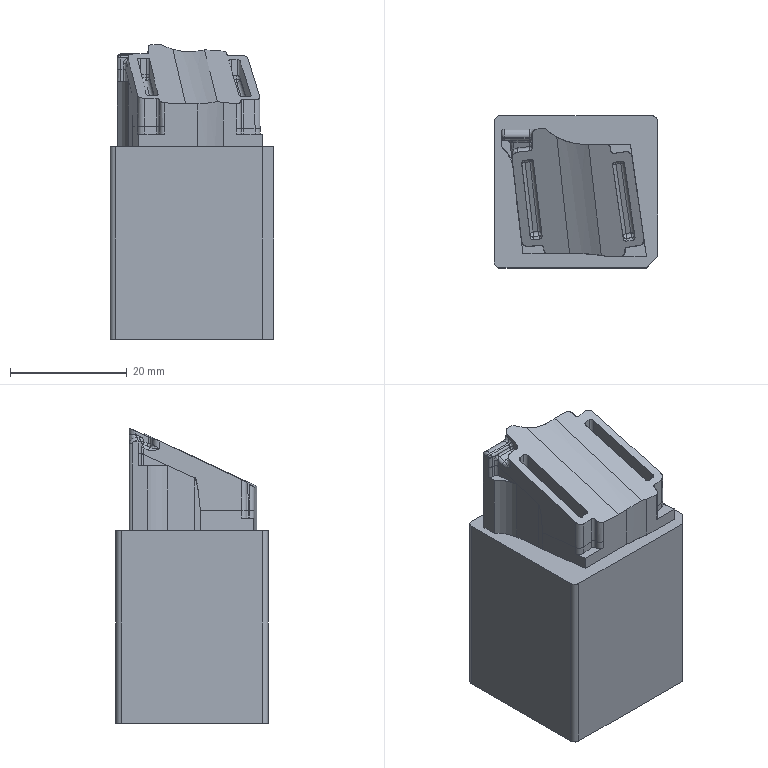NC program | NX | posted with a generic post | part box 28 x 26 x 50.455 mm
Lines 1 to 1102 of 7117:
N10 G17 G21 G94 G90
(ZLEVEL_PROFILE , TOOL : D0.8R0.4)
N12 T00 M6
N14 G54
N16 G17 G0 G90 X-7.861 Y4.615 S0 M3
N18 G43 Z10. H0
N20 Z-2.448
N22 G94 G1 Z-2.748 F250.
N24 G3 X-7.798 Y5.095 R0.5
N26 G1 X-7.942 Y5.081
N28 X-8.842 Y4.976
N30 G3 X-8.688 Y4.441 R0.5
N32 G1 Z-2.448
N34 G0 Z-2.051
N36 X-7.863 Y4.484
N38 Z-2.547
N40 G1 Z-2.847
N42 G3 X-7.703 Y5.073 R0.5
N44 G1 X-7.715 Y5.081
N46 X-7.782 Y5.097
N48 X-7.887 Y5.086
N50 X-8.843 Y4.975
N52 X-8.886 Y4.929
N54 G3 X-8.592 Y4.37 R0.5
N56 G1 Z-2.547
N58 G0 Z-2.448
N60 X-7.912 Y4.453
N62 Z-2.646
N64 G1 Z-2.946
N66 G3 X-7.676 Y5.041 R0.5
N68 G1 X-7.687 Y5.054
N70 X-7.719 Y5.083
N72 X-7.782 Y5.097
N74 X-7.831 Y5.092
N76 X-8.783 Y4.981
N78 X-8.853 Y4.965
N80 X-8.884 Y4.932
N82 X-8.888 Y4.921
N84 X-8.9 Y4.863
N86 G3 X-8.543 Y4.282 R0.5
N88 G1 Z-2.646
N90 G0 Z-2.547
N92 X-7.947 Y4.357
N94 Z-2.745
N96 G1 Z-3.045
N98 G3 X-7.646 Y4.876 R0.5
N100 G1 X-7.657 Y4.969
N102 X-7.673 Y5.038
N104 X-7.687 Y5.054
N106 X-7.719 Y5.083
N108 X-7.766 Y5.095
N110 X-7.799
N112 X-8.781 Y4.981
N114 X-8.854 Y4.964
N116 X-8.878 Y4.938
N118 X-8.899 Y4.827
N120 X-8.887 Y4.729
N122 X-8.882 Y4.647
N124 G3 X-8.481 Y4.193 R0.5
N126 G1 Z-2.745
N128 G0 Z-2.646
N130 X-7.899 Y4.108
N132 Z-2.845
N134 G1 Z-3.145
N136 G3 X-7.623 Y4.665 R0.5
N138 G2 X-7.646 Y4.872 R1.046
N140 G1 X-7.658 Y4.973
N142 X-7.673 Y5.038
N144 X-7.687 Y5.054
N146 X-7.709 Y5.074
N148 X-7.799 Y5.094
N150 X-8.779 Y4.98
N152 X-8.855 Y4.962
N154 X-8.878 Y4.938
N156 X-8.898 Y4.83
N158 X-8.873 Y4.607
N160 X-8.864 Y4.546
N162 G3 X-8.459 Y4.114 R0.5
N164 G1 Z-2.845
N166 G0 Z-2.745
N168 X-7.874 Y3.946
N170 Z-2.944
N172 G1 Z-3.244
N174 G3 X-7.597 Y4.454 R0.5
N176 G1 X-7.621 Y4.656
N178 G2 X-7.646 Y4.867 R1.046
N180 G1 X-7.659 Y4.978
N182 X-7.673 Y5.038
N184 X-7.687 Y5.054
N186 X-7.709 Y5.074
N188 X-7.782 Y5.09
N190 X-7.799 Y5.093
N192 X-8.778 Y4.979
N194 X-8.858 Y4.96
N196 X-8.878 Y4.938
N198 X-8.897 Y4.833
N200 X-8.871 Y4.595
N202 X-8.858 Y4.483
N204 X-8.838 Y4.306
N206 G3 X-8.445 Y3.872 R0.5
N208 G1 Z-2.944
N210 G0 Z-2.845
N212 X-7.867 Y3.726
N214 Z-3.043
N216 G1 Z-3.343
N218 G3 X-7.573 Y4.242 R0.5
N220 G1 X-7.622 Y4.661
N222 G2 X-7.646 Y4.861 R1.046
N224 G1 X-7.66 Y4.982
N226 X-7.673 Y5.038
N228 X-7.687 Y5.054
N230 X-7.709 Y5.074
N232 X-7.726 Y5.078
N234 X-7.799 Y5.092
N236 X-8.776 Y4.979
N238 X-8.86 Y4.957
N240 X-8.878 Y4.938
N242 X-8.897 Y4.836
N244 X-8.868 Y4.579
N246 X-8.859 Y4.499
N248 X-8.814 Y4.095
N250 G3 X-8.422 Y3.661 R0.5
N252 G1 Z-3.043
N254 G0 Z-2.944
N256 X-7.858 Y3.508
N258 Z-3.142
N260 G1 Z-3.442
N262 G3 X-7.548 Y4.031 R0.5
N264 G1 X-7.566 Y4.178
N266 X-7.57 Y4.217
N268 X-7.623 Y4.666
N270 X-7.646 Y4.856
N272 X-7.661 Y4.987
N274 X-7.673 Y5.038
N276 X-7.687 Y5.054
N278 X-7.707 Y5.072
N280 X-7.8 Y5.091
N282 X-8.774 Y4.978
N284 X-8.863 Y4.954
N286 X-8.878 Y4.938
N288 X-8.896 Y4.839
N290 X-8.864 Y4.548
N292 X-8.862 Y4.53
N294 X-8.789 Y3.883
N296 G3 X-8.392 Y3.449 R0.5
N298 G1 Z-3.142
N300 G0 Z-3.043
N302 X-7.808 Y3.275
N304 Z-3.241
N306 G1 Z-3.541
N308 G3 X-7.532 Y3.818 R0.5
N310 G2 X-7.548 Y4.028 R0.976
N312 G1 X-7.625 Y4.672
N314 X-7.646 Y4.85
N316 X-7.662 Y4.991
N318 X-7.672 Y5.037
N320 X-7.719 Y5.075
N322 X-7.797 Y5.09
N324 X-7.802
N326 X-8.78 Y4.976
N328 X-8.848 Y4.958
N330 X-8.887 Y4.89
N332 X-8.896 Y4.842
N334 X-8.765 Y3.672
N336 G3 X-8.362 Y3.236 R0.5
N338 G1 Z-3.241
N340 G0 Z-3.142
N342 X-7.793 Y3.092
N344 Z-3.341
N346 G1 Z-3.641
N348 G3 X-7.499 Y3.608 R0.5
N350 G1 X-7.515 Y3.745
N352 G2 X-7.548 Y4.024 R0.976
N354 G1 X-7.626 Y4.678
N356 X-7.645 Y4.844
N358 X-7.664 Y4.996
N360 X-7.672 Y5.035
N362 X-7.733 Y5.077
N364 X-7.789 Y5.089
N366 X-7.812 Y5.088
N368 X-8.778 Y4.976
N370 X-8.839 Y4.957
N372 X-8.859 Y4.94
N374 X-8.887 Y4.89
N376 X-8.895 Y4.848
N378 X-8.894 Y4.834
N380 X-8.74 Y3.461
N382 G3 X-8.338 Y3.025 R0.5
N384 G1 Z-3.341
N386 G0 Z-3.241
N388 X-7.763 Y2.884
N390 Z-3.44
N392 G1 Z-3.74
N394 G3 X-7.475 Y3.397 R0.5
N396 G1 X-7.516 Y3.749
N398 G2 X-7.548 Y4.02 R0.976
N400 G1 X-7.627 Y4.685
N402 X-7.645 Y4.837
N404 X-7.665 Y5.001
N406 X-7.672 Y5.033
N408 X-7.75 Y5.081
N410 X-7.776 Y5.086
N412 X-7.817
N414 X-8.77 Y4.976
N416 X-8.839 Y4.955
N418 X-8.862 Y4.934
N420 X-8.887 Y4.89
N422 X-8.894 Y4.853
N424 X-8.893 Y4.834
N426 X-8.716 Y3.249
N428 G3 X-8.319 Y2.815 R0.5
N430 G1 Z-3.44
N432 G0 Z-3.341
N434 X-7.735 Y2.674
N436 Z-3.539
N438 G1 Z-3.839
N440 G3 X-7.45 Y3.186 R0.5
N442 G1 X-7.517 Y3.753
N444 G2 X-7.549 Y4.017 R0.976
N446 G1 X-7.629 Y4.692
N448 X-7.645 Y4.829
N450 X-7.666 Y5.006
N452 X-7.671 Y5.03
N454 X-7.728 Y5.104
N456 X-7.819 Y5.085
N458 X-8.767 Y4.975
N460 X-8.838 Y4.953
N462 X-8.867 Y4.926
N464 X-8.884 Y4.895
N466 X-8.889 Y4.881
N468 X-8.892 Y4.861
N470 Y4.834
N472 X-8.691 Y3.038
N474 G3 X-8.31 Y2.607 R0.5
N476 G1 Z-3.539
N478 G0 Z-3.44
N480 X-7.716 Y2.46
N482 Z-3.638
N484 G1 Z-3.938
N486 G3 X-7.426 Y2.974 R0.5
N488 G1 X-7.518 Y3.756
N490 G2 X-7.549 Y4.013 R0.976
N492 G1 X-7.63 Y4.7
N494 X-7.644 Y4.821
N496 X-7.667 Y5.011
N498 X-7.671 Y5.028
N500 X-7.728 Y5.102
N502 X-7.821 Y5.084
N504 X-8.767 Y4.975
N506 X-8.837 Y4.951
N508 X-8.908 Y4.912
N510 X-8.891 Y4.833
N512 X-8.667 Y2.827
N514 G3 X-8.27 Y2.392 R0.5
N516 G1 Z-3.638
N518 G0 Z-3.539
N520 X-7.69 Y2.249
N522 Z-3.738
N524 G1 Z-4.038
N526 G3 X-7.401 Y2.763 R0.5
N528 G1 X-7.519 Y3.76
N530 G2 X-7.549 Y4.009 R0.976
N532 G1 X-7.632 Y4.71
N534 X-7.644 Y4.811
N536 X-7.668 Y5.016
N538 X-7.67 Y5.026
N540 X-7.729 Y5.101
N542 X-7.822 Y5.083
N544 X-8.766 Y4.974
N546 X-8.773 Y4.972
N548 X-8.805 Y4.962
N550 X-8.877 Y4.943
N552 X-8.913 Y4.877
N554 X-8.887 Y4.806
N556 X-8.642 Y2.615
N558 G3 X-8.243 Y2.181 R0.5
N560 G1 Z-3.738
N562 G0 Z-3.638
N564 X-7.666 Y2.038
N566 Z-3.837
N568 G1 Z-4.137
N570 G3 X-7.377 Y2.552 R0.5
N572 G1 X-7.52 Y3.764
N574 G2 X-7.549 Y4.005 R0.976
N576 G1 X-7.634 Y4.722
N578 X-7.643 Y4.799
N580 X-7.669 Y5.022
N582 X-7.67 Y5.026
N584 X-7.692 Y5.047
N586 X-7.801 Y5.082
N588 X-7.833 Y5.081
N590 X-8.767 Y4.973
N592 X-8.782 Y4.969
N594 X-8.796 Y4.965
N596 X-8.872 Y4.948
N598 X-8.911 Y4.88
N600 X-8.887 Y4.806
N602 X-8.618 Y2.404
N604 G3 X-8.221 Y1.97 R0.5
N606 G1 Z-3.837
N608 G0 Z-3.738
N610 X-7.647 Y1.824
N612 Z-3.936
N614 G1 Z-4.236
N616 G3 X-7.352 Y2.34 R0.5
N618 G1 X-7.521 Y3.768
N620 G2 X-7.549 Y4. R0.976
N622 G1 X-7.636 Y4.739
N624 X-7.641 Y4.781
N626 X-7.67 Y5.026
N628 X-7.69 Y5.045
N630 X-7.801 Y5.081
N632 X-7.835 Y5.08
N634 X-8.768 Y4.972
N636 G3 X-8.886 Y4.807 R0.144
N638 G1 X-8.593 Y2.193
N640 G3 X-8.195 Y1.758 R0.5
N642 G1 Z-3.936
N644 G0 Z-3.837
N646 X-7.642 Y1.605
N648 Z-4.035
N650 G1 Z-4.335
N652 G3 X-7.327 Y2.129 R0.5
N654 G1 X-7.344 Y2.27
N656 X-7.35 Y2.317
N658 X-7.522 Y3.773
N660 G2 X-7.549 Y3.996 R0.976
N662 G1 X-7.671 Y5.027
N664 X-7.69 Y5.045
N666 X-7.797 Y5.079
N668 X-7.836
N670 X-8.769 Y4.971
N672 G3 X-8.885 Y4.807 R0.142
N674 G1 X-8.569 Y1.981
N676 G3 X-8.154 Y1.544 R0.5
N678 G1 Z-4.035
N680 G0 Z-3.936
N682 X-7.588 Y1.379
N684 Z-4.134
N686 G1 Z-4.434
N688 G3 X-7.314 Y1.916 R0.5
N690 G2 X-7.328 Y2.126 R0.95
N692 G1 X-7.523 Y3.777
N694 G2 X-7.549 Y3.991 R0.976
N696 G1 X-7.671 Y5.028
N698 X-7.69 Y5.045
N700 X-7.792 Y5.078
N702 X-7.838
N704 X-8.769 Y4.97
N706 G3 X-8.884 Y4.808 R0.141
N708 G1 X-8.567 Y1.975
N710 G2 X-8.54 Y1.77 R1.012
N712 G3 X-8.133 Y1.293 R0.5
N714 G1 Z-4.134
N716 G0 Z-4.035
N718 X-7.574 Y1.19
N720 Z-4.234
N722 G1 Z-4.534
N724 G3 X-7.278 Y1.707 R0.5
N726 G1 X-7.289 Y1.795
N728 X-7.293 Y1.825
N730 G2 X-7.328 Y2.123 R0.95
N732 G1 X-7.524 Y3.782
N734 G2 X-7.549 Y3.986 R0.976
N736 G1 X-7.672 Y5.028
N738 X-7.69 Y5.045
N740 X-7.789 Y5.077
N742 X-7.839
N744 X-8.779 Y4.968
N746 X-8.848 Y4.967
N748 X-8.868 Y4.901
N750 X-8.883 Y4.839
N752 Y4.809
N754 X-8.565 Y1.968
N756 G2 X-8.54 Y1.752 R1.012
N758 G1 X-8.514 Y1.559
N760 G3 X-8.11 Y1.086 R0.5
N762 G1 Z-4.234
N764 G0 Z-4.134
N766 X-7.545 Y0.981
N768 Z-4.333
N770 G1 Z-4.633
N772 G3 X-7.254 Y1.495 R0.5
N774 G1 X-7.27 Y1.629
N776 X-7.276 Y1.685
N778 X-7.291 Y1.808
N780 X-7.293 Y1.825
N782 G2 X-7.328 Y2.12 R0.95
N784 G1 X-7.525 Y3.787
N786 X-7.549 Y3.981
N788 X-7.673 Y5.029
N790 X-7.687 Y5.043
N792 X-7.698 Y5.047
N794 X-7.789 Y5.077
N796 X-7.824 Y5.078
N798 X-8.785 Y4.966
N800 X-8.851 Y4.965
N802 X-8.868 Y4.901
N804 X-8.873 Y4.882
N806 X-8.883 Y4.81
N808 X-8.564 Y1.96
N810 G2 X-8.54 Y1.752 R1.012
N812 X-8.514 Y1.532 R0.996
N814 G1 X-8.491 Y1.348
N816 G3 X-8.096 Y0.873 R0.5
N818 G1 Z-4.333
N820 G0 Z-4.234
N822 X-7.518 Y0.77
N824 Z-4.432
N826 G1 Z-4.732
N828 G3 X-7.229 Y1.284 R0.5
N830 G1 X-7.294 Y1.826
N832 G2 X-7.328 Y2.116 R0.95
N834 G1 X-7.527 Y3.792
N836 X-7.548 Y3.976
N838 X-7.673 Y5.03
N840 X-7.686 Y5.041
N842 X-7.706 Y5.05
N844 X-7.789 Y5.077
N846 X-7.816 Y5.078
N848 X-8.74 Y4.971
N850 X-8.739 Y4.964
N852 X-8.811 Y4.956
N854 X-8.868 Y4.901
N856 X-8.873 Y4.882
N858 X-8.874 Y4.869
N860 X-8.882 Y4.811
N862 X-8.562 Y1.952
N864 X-8.54 Y1.755
N866 X-8.539 Y1.75
N868 G2 X-8.514 Y1.532 R0.996
N870 X-8.491 Y1.317 R1.013
N872 G1 X-8.471 Y1.136
N874 G3 X-8.085 Y0.704 R0.5
N876 G1 Z-4.432
N878 G0 Z-4.333
N880 X-7.497 Y0.557
N882 Z-4.531
N884 G1 Z-4.831
N886 G3 X-7.205 Y1.073 R0.5
N888 G1 X-7.295 Y1.829
N890 G2 X-7.328 Y2.113 R0.95
N892 G1 X-7.528 Y3.797
N894 X-7.548 Y3.97
N896 X-7.674 Y5.03
N898 X-7.684 Y5.04
N900 X-7.714 Y5.053
N902 X-7.789 Y5.077
N904 X-7.809 Y5.078
N906 X-8.74 Y4.97
N908 X-8.739 Y4.964
N910 X-8.811 Y4.956
N912 X-8.868 Y4.901
N914 X-8.871 Y4.887
N916 X-8.881 Y4.812
N918 X-8.56 Y1.942
N920 X-8.54 Y1.764
N922 X-8.538 Y1.743
N924 G2 X-8.514 Y1.532 R0.996
N926 X-8.491 Y1.325 R1.013
N928 G1 X-8.446 Y0.925
N930 G3 X-8.056 Y0.492 R0.5
N932 G1 Z-4.531
N934 G0 Z-4.432
N936 X-7.476 Y0.344
N938 Z-4.631
N940 G1 Z-4.931
N942 G3 X-7.18 Y0.861 R0.5
N944 G1 X-7.295 Y1.832
N946 G2 X-7.328 Y2.109 R0.95
N948 G1 X-7.529 Y3.803
N950 X-7.548 Y3.964
N952 X-7.674 Y5.031
N954 X-7.682 Y5.038
N956 X-7.724 Y5.056
N958 X-7.789 Y5.077
N960 X-7.803 Y5.078
N962 X-8.701 Y4.973
N964 Y4.969
N966 X-8.811 Y4.956
N968 X-8.868 Y4.901
N970 X-8.869 Y4.895
N972 X-8.879 Y4.804
N974 X-8.558 Y1.932
N976 X-8.54 Y1.774
N978 X-8.536 Y1.735
N980 G2 X-8.514 Y1.535 R0.996
N982 G1 X-8.513 Y1.529
N984 X-8.491 Y1.333
N986 X-8.424 Y0.738
N988 G3 X-8.019 Y0.302 R0.5
N990 G1 Z-4.631
N992 G0 Z-4.531
N994 X-7.436 Y0.141
N996 Z-4.73
N998 G1 Z-5.03
N1000 G3 X-7.156 Y0.65 R0.5
N1002 G1 X-7.296 Y1.836
N1004 G2 X-7.328 Y2.106 R0.95
N1006 G1 X-7.53 Y3.81
N1008 X-7.548 Y3.958
N1010 X-7.675 Y5.031
N1012 X-7.68 Y5.036
N1014 X-7.771 Y5.071
N1016 X-7.784 Y5.075
N1018 X-8.811 Y4.956
N1020 X-8.867 Y4.902
N1022 X-8.878 Y4.796
N1024 X-8.556 Y1.921
N1026 X-8.541 Y1.786
N1028 X-8.534 Y1.726
N1030 X-8.514 Y1.544
N1032 X-8.511 Y1.52
N1034 X-8.491 Y1.343
N1036 X-8.397 Y0.502
N1038 G3 X-8.004 Y0.069 R0.5
N1040 G1 Z-4.73
N1042 G0 Z-4.631
N1044 X-7.417 Y-0.073
N1046 Z-4.829
N1048 G1 Z-5.129
N1050 G3 X-7.131 Y0.439 R0.5
N1052 G1 X-7.297 Y1.839
N1054 G2 X-7.328 Y2.102 R0.95
N1056 G1 X-7.532 Y3.817
N1058 X-7.548 Y3.951
N1060 X-7.676 Y5.032
N1062 X-7.68 Y5.036
N1064 X-7.682 Y5.037
N1066 X-7.771 Y5.071
N1068 X-7.784 Y5.075
N1070 X-8.811 Y4.956
N1072 X-8.857 Y4.918
N1074 X-8.877 Y4.796
N1076 X-8.553 Y1.906
N1078 X-8.542 Y1.801
N1080 X-8.532 Y1.716
N1082 X-8.514 Y1.554
N1084 X-8.509 Y1.509
N1086 X-8.491 Y1.353
N1088 X-8.373 Y0.291
N1090 G3 X-7.976 Y-0.143 R0.5
N1092 G1 Z-4.829
N1094 G0 Z-4.73
N1096 X-7.42 Y-0.297
N1098 Z-4.928
N1100 G1 Z-5.228
N1102 G3 X-7.107 Y0.227 R0.5
N1104 G1 X-7.298 Y1.843
N1106 G2 X-7.329 Y2.098 R0.95
N1108 G1 X-7.533 Y3.825
N1110 X-7.547 Y3.943
N1112 X-7.676 Y5.033
N1114 X-7.678 Y5.034
N1116 X-7.687 Y5.039
N1118 X-7.771 Y5.071
N1120 X-7.784 Y5.075
N1122 X-8.811 Y4.956
N1124 X-8.856 Y4.918
N1126 X-8.876 Y4.795
N1128 X-8.55 Y1.886
N1130 X-8.543 Y1.821
N1132 X-8.53 Y1.705
N1134 X-8.514 Y1.565
N1136 X-8.507 Y1.497
N1138 X-8.492 Y1.365
N1140 X-8.349 Y0.083
N1142 G3 X-7.931 Y-0.355 R0.5
N1144 G1 Z-4.928
N1146 G0 Z-4.829
N1148 X-7.367 Y-0.526
N1150 Z-5.028
N1152 G1 Z-5.328
N1154 G3 X-7.092 Y0.014 R0.5
N1156 G2 X-7.107 Y0.224 R0.961
N1158 G1 X-7.299 Y1.847
N1160 G2 X-7.329 Y2.094 R0.95
N1162 G1 X-7.535 Y3.834
N1164 X-7.547 Y3.934
N1166 X-7.677 Y5.033
N1168 X-7.693 Y5.041
N1170 X-7.771 Y5.071
N1172 X-7.784 Y5.075
N1174 X-8.811 Y4.956
N1176 X-8.856 Y4.918
N1178 X-8.873 Y4.812
N1180 X-8.847 Y4.587
N1182 X-8.852
N1184 X-8.528 Y1.692
N1186 X-8.515 Y1.579
N1188 X-8.504 Y1.483
N1190 X-8.493 Y1.38
N1192 X-8.347 Y0.077
N1194 G2 X-8.318 Y-0.132 R1.003
N1196 G3 X-7.917 Y-0.606 R0.5
N1198 G1 Z-5.028
N1200 G0 Z-4.928
N1202 X-7.345 Y-0.708
N1204 Z-5.127
N1206 G1 Z-5.427
N1208 G3 X-7.058 Y-0.195 R0.5
N1210 G1 X-7.072 Y-0.073
N1212 G2 X-7.107 Y0.221 R0.961
N1214 G1 X-7.3 Y1.851
N1216 G2 X-7.329 Y2.09 R0.95
N1218 G1 X-7.537 Y3.845
N1220 X-7.546 Y3.922
N1222 X-7.677 Y5.032
N1224 X-7.698 Y5.043
N1226 X-7.771 Y5.071
N1228 X-7.784 Y5.075
N1230 X-8.811 Y4.956
N1232 X-8.856 Y4.918
N1234 X-8.873 Y4.812
N1236 X-8.842 Y4.547
N1238 X-8.846 Y4.546
N1240 X-8.525 Y1.674
N1242 X-8.516 Y1.597
N1244 X-8.501 Y1.462
N1246 X-8.494 Y1.401
N1248 X-8.345 Y0.07
N1250 G2 X-8.318 Y-0.158 R1.003
N1252 G1 X-8.297 Y-0.343
N1254 G3 X-7.906 Y-0.82 R0.5
N1256 G1 Z-5.127
N1258 G0 Z-5.028
N1260 X-7.323 Y-0.921
N1262 Z-5.226
N1264 G1 Z-5.526
N1266 G3 X-7.033 Y-0.407 R0.5
N1268 G1 X-7.073 Y-0.07
N1270 G2 X-7.107 Y0.217 R0.961
N1272 G1 X-7.301 Y1.855
N1274 G2 X-7.329 Y2.086 R0.95
N1276 G1 X-7.539 Y3.861
N1278 X-7.544 Y3.906
N1280 X-7.678 Y5.031
N1282 X-7.785 Y5.075
N1284 X-8.811 Y4.956
N1286 X-8.856 Y4.918
N1288 X-8.873 Y4.812
N1290 X-8.842 Y4.547
N1292 X-8.845 Y4.546
N1294 X-8.344 Y0.063
N1296 G2 X-8.318 Y-0.158 R1.003
N1298 X-8.297 Y-0.357 R1.03
N1300 G1 X-8.275 Y-0.554
N1302 G3 X-7.871 Y-0.99 R0.5
N1304 G1 Z-5.226
N1306 G0 Z-5.127
N1308 X-7.3 Y-1.133
N1310 Z-5.325
N1312 G1 Z-5.625
N1314 G3 X-7.009 Y-0.618 R0.5
N1316 G1 X-7.074 Y-0.066
N1318 G2 X-7.107 Y0.214 R0.961
N1320 G1 X-7.302 Y1.859
N1322 G2 X-7.329 Y2.082 R0.95
N1324 G1 X-7.678 Y5.03
N1326 X-7.787 Y5.074
N1328 X-8.811 Y4.956
N1330 X-8.856 Y4.918
N1332 X-8.873 Y4.812
N1334 X-8.842 Y4.547
N1336 X-8.844
N1338 X-8.342 Y0.056
N1340 G2 X-8.318 Y-0.158 R1.003
N1342 G1 X-8.297 Y-0.348
N1344 X-8.25 Y-0.766
N1346 G3 X-7.856 Y-1.199 R0.5
N1348 G1 Z-5.325
N1350 G0 Z-5.226
N1352 X-7.285 Y-1.348
N1354 Z-5.424
N1356 G1 Z-5.724
N1358 G3 X-6.984 Y-0.829 R0.5
N1360 G1 X-7.075 Y-0.063
N1362 G2 X-7.107 Y0.21 R0.961
N1364 G1 X-7.303 Y1.863
N1366 G2 X-7.329 Y2.077 R0.95
N1368 G1 X-7.678 Y5.029
N1370 X-7.79 Y5.074
N1372 X-8.811 Y4.956
N1374 X-8.856 Y4.918
N1376 X-8.873 Y4.812
N1378 X-8.842 Y4.547
N1380 X-8.844
N1382 X-8.34 Y0.048
N1384 G2 X-8.318 Y-0.152 R1.003
N1386 G1 X-8.316 Y-0.165
N1388 X-8.297 Y-0.339
N1390 X-8.226 Y-0.977
N1392 G3 X-7.826 Y-1.412 R0.5
N1394 G1 Z-5.424
N1396 G0 Z-5.325
N1398 X-7.294 Y-1.411
N1400 Z-5.524
N1402 G1 Z-5.824
N1404 G3 X-6.981 Y-0.907 R0.5
N1406 G1 X-6.984 Y-0.834
N1408 X-7.076 Y-0.059
N1410 G2 X-7.108 Y0.207 R0.961
N1412 G1 X-7.304 Y1.868
N1414 G2 X-7.329 Y2.073 R0.95
N1416 G1 X-7.676 Y5.003
N1418 X-7.709 Y5.041
N1420 X-7.79 Y5.074
N1422 X-8.811 Y4.956
N1424 X-8.856 Y4.918
N1426 X-8.857 Y4.916
N1428 X-8.873 Y4.812
N1430 X-8.842 Y4.547
N1432 X-8.832 Y4.45
N1434 X-8.338 Y0.039
N1436 X-8.318 Y-0.143
N1438 X-8.314 Y-0.176
N1440 X-8.297 Y-0.328
N1442 X-8.201 Y-1.188
N1444 G3 X-7.803 Y-1.623 R0.5
N1446 G1 Z-5.524
N1448 G0 Z-5.424
N1450 X-7.255 Y-1.659
N1452 Z-5.623
N1454 G1 Z-5.923
N1456 G3 X-6.949 Y-1.137 R0.5
N1458 G1 X-6.959 Y-1.052
N1460 G2 X-6.984 Y-0.839 R1.044
N1462 G1 X-7.077 Y-0.056
N1464 G2 X-7.108 Y0.203 R0.961
N1466 G1 X-7.305 Y1.873
N1468 X-7.329 Y2.068
N1470 X-7.611 Y4.45
N1472 X-7.626 Y4.578
N1474 X-7.65 Y4.786
N1476 X-7.676 Y5.003
N1478 X-7.7 Y5.031
N1480 X-7.71 Y5.042
N1482 X-7.79 Y5.074
N1484 X-8.811 Y4.956
N1486 X-8.855 Y4.919
N1488 X-8.857 Y4.912
N1490 X-8.873 Y4.812
N1492 X-8.829 Y4.434
N1494 X-8.336 Y0.029
N1496 X-8.318 Y-0.133
N1498 X-8.312 Y-0.188
N1500 X-8.298 Y-0.315
N1502 X-8.177 Y-1.393
N1504 G3 X-7.779 Y-1.827 R0.5
N1506 G1 Z-5.623
N1508 G0 Z-5.524
N1510 X-7.199 Y-1.977
N1512 Z-5.722
N1514 G1 Z-6.022
N1516 G3 X-6.911 Y-1.463 R0.5
N1518 G1 X-6.96 Y-1.047
N1520 G2 X-6.984 Y-0.844 R1.044
N1522 G1 X-7.078 Y-0.052
N1524 G2 X-7.108 Y0.199 R0.961
N1526 G1 X-7.307 Y1.878
N1528 X-7.329 Y2.063
N1530 X-7.601 Y4.364
N1532 X-7.65 Y4.786
N1534 X-7.676 Y5.003
N1536 X-7.692 Y5.022
N1538 X-7.71 Y5.042
N1540 X-7.79 Y5.074
N1542 X-8.811 Y4.956
N1544 X-8.855 Y4.92
N1546 X-8.858 Y4.907
N1548 X-8.873 Y4.812
N1550 X-8.805 Y4.222
N1552 X-8.334 Y0.018
N1554 X-8.319 Y-0.122
N1556 X-8.309 Y-0.204
N1558 X-8.299 Y-0.299
N1560 X-8.152 Y-1.611
N1562 G3 X-7.755 Y-2.045 R0.5
N1564 G1 Z-5.722
N1566 G0 Z-5.623
N1568 X-7.198 Y-2.198
N1570 Z-5.821
N1572 G1 Z-6.121
N1574 G3 X-6.886 Y-1.675 R0.5
N1576 G1 X-6.961 Y-1.042
N1578 X-6.984 Y-0.85
N1580 X-7.079 Y-0.048
N1582 G2 X-7.108 Y0.195 R0.961
N1584 G1 X-7.308 Y1.883
N1586 X-7.328 Y2.057
N1588 X-7.577 Y4.153
N1590 X-7.65 Y4.786
N1592 X-7.676 Y5.003
N1594 X-7.692 Y5.022
N1596 X-7.71 Y5.042
N1598 X-7.78 Y5.07
N1600 X-7.818 Y5.071
N1602 X-8.72 Y4.966
N1604 X-8.812 Y4.947
N1606 X-8.855 Y4.918
N1608 X-8.858 Y4.907
N1610 X-8.873 Y4.812
N1612 X-8.78 Y4.011
N1614 X-8.332 Y0.004
N1616 X-8.319 Y-0.108
N1618 X-8.306 Y-0.229
N1620 X-8.301 Y-0.273
N1622 X-8.127 Y-1.822
N1624 G3 X-7.712 Y-2.26 R0.5
N1626 G1 Z-5.821
N1628 G0 Z-5.722
N1630 X-7.201 Y-2.244
N1632 Z-5.921
N1634 G1 Z-6.221
N1636 G3 X-6.886 Y-1.756 R0.5
N1638 G1 Y-1.678
N1640 X-6.962 Y-1.036
N1642 X-6.984 Y-0.855
N1644 X-7.08 Y-0.044
N1646 G2 X-7.108 Y0.191 R0.961
N1648 G1 X-7.309 Y1.889
N1650 X-7.328 Y2.051
N1652 X-7.552 Y3.941
N1654 X-7.64 Y4.697
N1656 G3 X-7.746 Y4.974 R0.595
N1658 G1 X-7.778 Y5.017
N1660 X-7.818 Y5.041
N1662 X-8.682 Y4.941
N1664 G3 X-8.83 Y4.778 R0.168
N1666 G1 X-8.838 Y4.506
N1668 X-8.756 Y3.8
N1670 X-8.329 Y-0.014
N1672 X-8.32 Y-0.09
N1674 X-8.126 Y-1.829
N1676 G2 X-8.099 Y-2.033 R1.012
N1678 G3 X-7.696 Y-2.51 R0.5
N1680 G1 Z-5.921
N1682 G0 Z-5.821
N1684 X-7.127 Y-2.611
N1686 Z-6.02
N1688 G1 Z-6.32
N1690 G3 X-6.837 Y-2.097 R0.5
N1692 G1 X-6.852 Y-1.969
N1694 G2 X-6.886 Y-1.681 R0.967
N1696 G1 X-6.964 Y-1.03
N1698 X-6.984 Y-0.862
N1700 X-7.081 Y-0.04
N1702 G2 X-7.108 Y0.186 R0.961
N1704 G1 X-7.31 Y1.895
N1706 X-7.328 Y2.045
N1708 X-7.528 Y3.73
N1710 X-7.612 Y4.456
N1712 G3 X-7.817 Y4.905 R0.801
N1714 G1 X-8.636 Y4.81
N1716 X-8.703 Y4.788
N1718 X-8.743 Y4.756
N1720 G3 X-8.812 Y4.287 R0.932
N1722 G1 X-8.732 Y3.593
N1724 X-8.711 Y3.404
N1726 X-8.124 Y-1.836
N1728 G2 X-8.099 Y-2.053 R1.012
N1730 G1 X-8.076 Y-2.245
N1732 G3 X-7.68 Y-2.722 R0.5
N1734 G1 Z-6.02
N1736 G0 Z-5.921
N1738 X-7.106 Y-2.824
N1740 Z-6.119
N1742 G1 Z-6.419
N1744 G3 X-6.813 Y-2.309 R0.5
N1746 G1 X-6.853 Y-1.966
N1748 G2 X-6.887 Y-1.685 R0.967
N1750 G1 X-6.965 Y-1.024
N1752 X-6.983 Y-0.868
N1754 X-7.082 Y-0.036
N1756 G2 X-7.108 Y0.182 R0.961
N1758 G1 X-7.311 Y1.901
N1760 X-7.328 Y2.038
N1762 X-7.503 Y3.519
N1764 X-7.573 Y4.122
N1766 X-7.663 Y4.517
N1768 G3 X-7.854 Y4.686 R0.227
N1770 G1 X-8.649 Y4.594
N1772 Z-6.416
N1774 X-8.66 Y4.693 Z-6.369
N1776 X-8.635 Y4.697 Z-6.372
N1778 X-7.877 Y4.797 Z-6.367
N1780 X-7.859 Y4.799 Z-6.364
N1782 X-7.848 Y4.786 Z-6.37
N1784 X-7.866 Z-6.371
N1786 X-7.876 Y4.784 Z-6.372
N1788 X-8.635 Y4.696
N1790 X-8.66 Y4.693 Z-6.369
N1792 X-8.649 Y4.594 Z-6.416
N1794 Z-6.419
N1796 X-8.665 Y4.592
N1798 G3 X-8.798 Y4.165 R0.655
N1800 G1 X-8.707 Y3.377
N1802 X-8.122 Y-1.844
N1804 G2 X-8.099 Y-2.053 R1.012
N1806 X-8.075 Y-2.265 R1.023
N1808 G1 X-8.064 Y-2.364
N1810 X-8.054 Y-2.456
N1812 G3 X-7.652 Y-2.892 R0.5
N1814 G1 Z-6.119
N1816 G0 Z-6.02
N1818 X-7.066 Y-3.028
N1820 Z-6.218
N1822 G1 Z-6.518
N1824 G3 X-6.788 Y-2.52 R0.5
N1826 G1 X-6.854 Y-1.962
N1828 G2 X-6.887 Y-1.688 R0.967
N1830 G1 X-6.966 Y-1.016
N1832 X-6.983 Y-0.875
N1834 X-7.083 Y-0.031
N1836 G2 X-7.108 Y0.177 R0.961
N1838 G1 X-7.313 Y1.909
N1840 X-7.327 Y2.031
N1842 X-7.479 Y3.307
N1844 X-7.558 Y3.995
N1846 X-7.663 Y4.357
N1848 X-7.847 Y4.473
N1850 X-8.591 Y4.387
N1852 X-8.605 Y4.435 Z-6.495
N1854 X-8.618 Y4.483 Z-6.471
N1856 X-8.611 Y4.494 Z-6.467
N1858 X-8.609 Y4.498 Z-6.466
N1860 X-7.857 Y4.585
N1862 X-7.852 Y4.584
N1864 X-7.813 Y4.567 Z-6.472
N1866 X-7.851 Y4.573
N1868 X-7.859 Y4.572
N1870 X-8.602 Y4.486
N1872 X-8.611 Y4.485
N1874 X-8.618 Y4.483 Z-6.471
N1876 X-8.605 Y4.435 Z-6.495
N1878 X-8.591 Y4.387 Z-6.518
N1880 G3 X-8.758 Y4.159 R0.231
N1882 G1 X-8.764 Y4.077
N1884 X-8.766 Y4.013
N1886 X-8.765 Y3.908
N1888 X-8.763 Y3.859
N1890 X-8.707 Y3.377
N1892 X-8.683 Y3.17
N1894 X-8.682 Y3.161
N1896 X-8.121 Y-1.852
N1898 X-8.099 Y-2.049
N1900 X-8.098 Y-2.057
N1902 G2 X-8.075 Y-2.257 R1.023
N1904 G1 X-8.071 Y-2.298
N1906 X-8.067 Y-2.33
N1908 X-8.029 Y-2.668
N1910 G3 X-7.636 Y-3.101 R0.5
N1912 G1 Z-6.218
N1914 G0 Z-6.119
N1916 X-7.049 Y-3.243
N1918 Z-6.318
N1920 G1 Z-6.618
N1922 G3 X-6.764 Y-2.731 R0.5
N1924 G1 X-6.855 Y-1.959
N1926 G2 X-6.887 Y-1.692 R0.967
N1928 G1 X-6.968 Y-1.008
N1930 X-6.983 Y-0.884
N1932 X-7.084 Y-0.026
N1934 G2 X-7.108 Y0.172 R0.961
N1936 G1 X-7.314 Y1.917
N1938 X-7.327 Y2.022
N1940 X-7.444 Y3.013
N1942 X-7.454 Y3.099
N1944 X-7.528 Y3.729
N1946 X-7.537 Y3.795
N1948 X-7.626 Y4.115
N1950 G3 X-7.822 Y4.262 R0.207
N1952 G1 X-8.567 Y4.175
N1954 X-8.577 Y4.196 Z-6.608
N1956 X-8.612 Y4.265 Z-6.57
N1958 X-8.587 Y4.281 Z-6.567
N1960 X-8.57 Y4.288 Z-6.565
N1962 X-7.871 Y4.37
N1964 X-7.854 Y4.359 Z-6.571
N1966 X-8.578 Y4.275
N1968 X-8.586 Y4.273
N1970 X-8.612 Y4.265 Z-6.57
N1972 X-8.577 Y4.196 Z-6.608
N1974 X-8.567 Y4.175 Z-6.618
N1976 G3 X-8.749 Y3.745 R0.557
N1978 G1 X-8.658 Y2.954
N1980 X-8.119 Y-1.861
N1982 X-8.099 Y-2.039
N1984 X-8.096 Y-2.066
N1986 X-8.075 Y-2.248
N1988 X-8.008 Y-2.854
N1990 G3 X-7.616 Y-3.287 R0.5
N1992 G1 Z-6.318
N1994 G0 Z-6.218
N1996 X-7.027 Y-3.456
N1998 Z-6.417
N2000 G1 Z-6.717
N2002 G3 X-6.739 Y-2.943 R0.5
N2004 G1 X-6.856 Y-1.955
N2006 G2 X-6.887 Y-1.696 R0.967
N2008 G1 X-6.969 Y-0.999
N2010 X-6.982 Y-0.893
N2012 X-7.085 Y-0.021
N2014 X-7.108 Y0.167
N2016 X-7.316 Y1.928
N2018 X-7.326 Y2.012
N2020 X-7.43 Y2.885
N2022 X-7.516 Y3.63
N2024 G3 X-7.629 Y3.918 R0.838
N2026 X-7.779 Y4.052 R0.134
N2028 G1 X-8.523 Y3.966
N2030 X-8.535 Y4.065 Z-6.67
N2032 X-8.522 Y4.08 Z-6.664
N2034 X-7.818 Y4.161
N2036 X-7.804 Y4.16 Z-6.666
N2038 X-7.781 Y4.153 Z-6.667
N2040 X-7.791 Y4.152 Z-6.669
N2042 X-7.802 Y4.15 Z-6.67
N2044 X-8.535 Y4.065
N2046 X-8.523 Y3.966 Z-6.717
N2048 X-8.539 Y3.964
N2050 X-8.605 Y3.947
N2052 G3 X-8.718 Y3.476 R0.802
N2054 G1 X-8.633 Y2.743
N2056 X-8.117 Y-1.872
N2058 X-8.099 Y-2.029
N2060 X-8.094 Y-2.076
N2062 X-8.076 Y-2.238
N2064 X-7.98 Y-3.09
N2066 G3 X-7.583 Y-3.525 R0.5
N2068 G1 Z-6.417
N2070 G0 Z-6.318
N2072 X-7.003 Y-3.667
N2074 Z-6.516
N2076 G1 Z-6.816
N2078 G3 X-6.715 Y-3.154 R0.5
N2080 G1 X-6.857 Y-1.951
N2082 G2 X-6.887 Y-1.7 R0.967
N2084 G1 X-6.971 Y-0.988
N2086 X-6.981 Y-0.904
N2088 X-7.086 Y-0.016
N2090 X-7.107 Y0.162
N2092 X-7.318 Y1.941
N2094 X-7.325 Y1.998
N2096 X-7.405 Y2.671
N2098 Y2.676
N2100 X-7.475 Y3.276
N2102 X-7.483 Y3.347
N2104 G3 X-7.663 Y3.813 R1.133
N2106 G1 X-7.774 Y3.839
N2108 X-8.533 Y3.751
N2110 X-8.544 Y3.85 Z-6.768
N2112 X-8.539 Y3.861 Z-6.765
N2114 X-8.52 Y3.866 Z-6.763
N2116 X-7.779 Y3.952
N2118 X-7.768 Y3.953 Z-6.762
N2120 X-7.732 Y3.932 Z-6.769
N2122 X-7.751 Y3.936
N2124 X-7.778 Y3.939
N2126 X-7.785 Y3.938
N2128 X-8.537 Y3.851
N2130 X-8.544 Y3.85 Z-6.768
N2132 X-8.533 Y3.751 Z-6.815
N2134 X-8.588 Y3.744 Z-6.816
N2136 G3 X-8.688 Y3.216 R0.926
N2138 G1 X-8.609 Y2.532
N2140 X-8.115 Y-1.883
N2142 X-8.1 Y-2.017
N2144 X-8.092 Y-2.087
N2146 X-8.076 Y-2.226
N2148 X-7.956 Y-3.302
N2150 G3 X-7.533 Y-3.74 R0.5
N2152 G1 Z-6.516
N2154 G0 Z-6.417
N2156 X-7.003 Y-3.889
N2158 Z-6.615
N2160 G1 Z-6.915
N2162 G3 X-6.69 Y-3.365 R0.5
N2164 G1 X-6.858 Y-1.947
N2166 G2 X-6.887 Y-1.704 R0.967
N2168 G1 X-6.974 Y-0.973
N2170 X-6.98 Y-0.92
N2172 X-7.088 Y-0.01
N2174 X-7.107 Y0.156
N2176 X-7.38 Y2.459
N2178 X-7.381 Y2.465
N2180 X-7.471 Y3.242
N2182 G3 X-7.749 Y3.628 R0.582
N2184 G1 X-8.493 Y3.541
N2186 X-8.505 Y3.641 Z-6.869
N2188 X-8.512 Y3.64
N2190 X-8.529 Y3.635 Z-6.868
N2192 X-8.522 Y3.651 Z-6.862
N2194 X-8.513 Y3.652 Z-6.863
N2196 X-7.78 Y3.738
N2198 X-7.754 Y3.731 Z-6.867
N2200 X-7.732 Y3.726 Z-6.868
N2202 X-7.753 Y3.728 Z-6.869